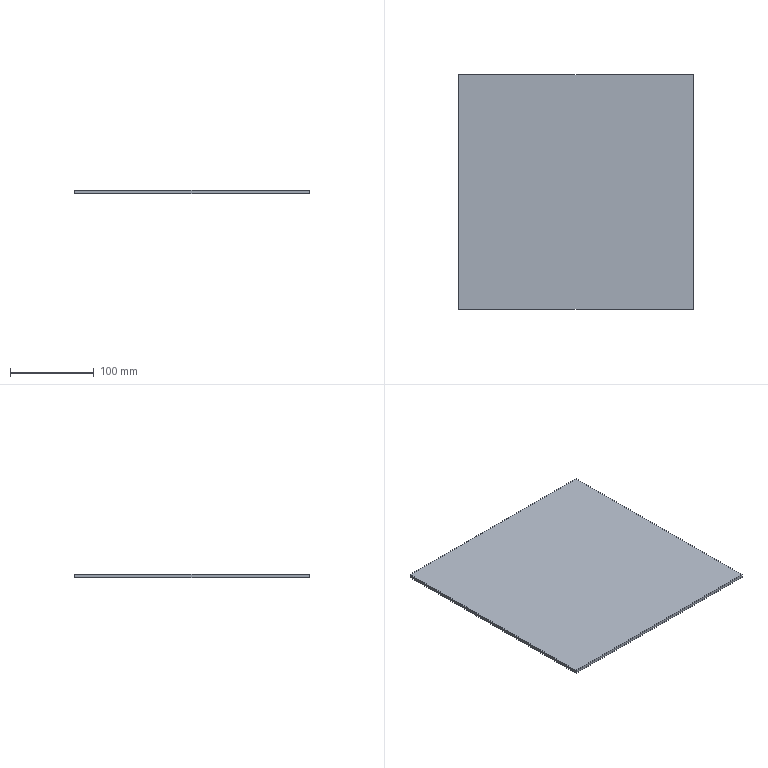Part | SolidWorks | features Extrusion 1 | 1 solid | 6 faces | box 280 x 280 x 4 mm | volume 313600 mm3 | plane 6
STEP:
#1=CARTESIAN_POINT('',(-140.,140.,2.));
#2=VERTEX_POINT('',#1);
#3=CARTESIAN_POINT('',(-140.,-140.,2.));
#4=VERTEX_POINT('',#3);
#5=CARTESIAN_POINT('',(-140.,140.,2.));
#6=DIRECTION('',(0.,-1.,0.));
#7=VECTOR('',#6,1000.);
#8=LINE('',#5,#7);
#9=EDGE_CURVE('',#2,#4,#8,.T.);
#10=ORIENTED_EDGE('',*,*,#9,.F.);
#11=CARTESIAN_POINT('',(-140.,140.,-2.));
#12=VERTEX_POINT('',#11);
#13=CARTESIAN_POINT('',(-140.,140.,-2.));
#14=DIRECTION('',(0.,0.,1.));
#15=VECTOR('',#14,1000.);
#16=LINE('',#13,#15);
#17=EDGE_CURVE('',#12,#2,#16,.T.);
#18=ORIENTED_EDGE('',*,*,#17,.F.);
#19=CARTESIAN_POINT('',(-140.,-140.,-2.));
#20=VERTEX_POINT('',#19);
#21=CARTESIAN_POINT('',(-140.,140.,-2.));
#22=DIRECTION('',(0.,-1.,0.));
#23=VECTOR('',#22,1000.);
#24=LINE('',#21,#23);
#25=EDGE_CURVE('',#12,#20,#24,.T.);
#26=ORIENTED_EDGE('',*,*,#25,.T.);
#27=CARTESIAN_POINT('',(-140.,-140.,-2.));
#28=DIRECTION('',(0.,0.,1.));
#29=VECTOR('',#28,1000.);
#30=LINE('',#27,#29);
#31=EDGE_CURVE('',#20,#4,#30,.T.);
#32=ORIENTED_EDGE('',*,*,#31,.T.);
#33=EDGE_LOOP('',(#10,#18,#26,#32));
#34=FACE_OUTER_BOUND('',#33,.T.);
#35=CARTESIAN_POINT('',(-140.,140.,-2.));
#36=DIRECTION('',(-1.,0.,0.));
#37=DIRECTION('',(0.,0.,1.));
#38=AXIS2_PLACEMENT_3D('',#35,#36,#37);
#39=PLANE('',#38);
#40=ADVANCED_FACE('',(#34),#39,.T.);
#41=CARTESIAN_POINT('',(140.,140.,2.));
#42=VERTEX_POINT('',#41);
#43=CARTESIAN_POINT('',(140.,140.,2.));
#44=DIRECTION('',(-1.,0.,0.));
#45=VECTOR('',#44,1000.);
#46=LINE('',#43,#45);
#47=EDGE_CURVE('',#42,#2,#46,.T.);
#48=ORIENTED_EDGE('',*,*,#47,.F.);
#49=CARTESIAN_POINT('',(140.,140.,-2.));
#50=VERTEX_POINT('',#49);
#51=CARTESIAN_POINT('',(140.,140.,-2.));
#52=DIRECTION('',(0.,0.,1.));
#53=VECTOR('',#52,1000.);
#54=LINE('',#51,#53);
#55=EDGE_CURVE('',#50,#42,#54,.T.);
#56=ORIENTED_EDGE('',*,*,#55,.F.);
#57=CARTESIAN_POINT('',(140.,140.,-2.));
#58=DIRECTION('',(-1.,0.,0.));
#59=VECTOR('',#58,1000.);
#60=LINE('',#57,#59);
#61=EDGE_CURVE('',#50,#12,#60,.T.);
#62=ORIENTED_EDGE('',*,*,#61,.T.);
#63=ORIENTED_EDGE('',*,*,#17,.T.);
#64=EDGE_LOOP('',(#48,#56,#62,#63));
#65=FACE_OUTER_BOUND('',#64,.T.);
#66=CARTESIAN_POINT('',(140.,140.,-2.));
#67=DIRECTION('',(0.,1.,0.));
#68=DIRECTION('',(0.,0.,1.));
#69=AXIS2_PLACEMENT_3D('',#66,#67,#68);
#70=PLANE('',#69);
#71=ADVANCED_FACE('',(#65),#70,.T.);
#72=CARTESIAN_POINT('',(140.,-140.,2.));
#73=VERTEX_POINT('',#72);
#74=CARTESIAN_POINT('',(140.,-140.,2.));
#75=DIRECTION('',(0.,1.,0.));
#76=VECTOR('',#75,1000.);
#77=LINE('',#74,#76);
#78=EDGE_CURVE('',#73,#42,#77,.T.);
#79=ORIENTED_EDGE('',*,*,#78,.F.);
#80=CARTESIAN_POINT('',(140.,-140.,-2.));
#81=VERTEX_POINT('',#80);
#82=CARTESIAN_POINT('',(140.,-140.,-2.));
#83=DIRECTION('',(0.,0.,1.));
#84=VECTOR('',#83,1000.);
#85=LINE('',#82,#84);
#86=EDGE_CURVE('',#81,#73,#85,.T.);
#87=ORIENTED_EDGE('',*,*,#86,.F.);
#88=CARTESIAN_POINT('',(140.,-140.,-2.));
#89=DIRECTION('',(0.,1.,0.));
#90=VECTOR('',#89,1000.);
#91=LINE('',#88,#90);
#92=EDGE_CURVE('',#81,#50,#91,.T.);
#93=ORIENTED_EDGE('',*,*,#92,.T.);
#94=ORIENTED_EDGE('',*,*,#55,.T.);
#95=EDGE_LOOP('',(#79,#87,#93,#94));
#96=FACE_OUTER_BOUND('',#95,.T.);
#97=CARTESIAN_POINT('',(140.,-140.,-2.));
#98=DIRECTION('',(1.,0.,0.));
#99=DIRECTION('',(0.,0.,-1.));
#100=AXIS2_PLACEMENT_3D('',#97,#98,#99);
#101=PLANE('',#100);
#102=ADVANCED_FACE('',(#96),#101,.T.);
#103=CARTESIAN_POINT('',(-140.,-140.,2.));
#104=DIRECTION('',(1.,0.,0.));
#105=VECTOR('',#104,1000.);
#106=LINE('',#103,#105);
#107=EDGE_CURVE('',#4,#73,#106,.T.);
#108=ORIENTED_EDGE('',*,*,#107,.F.);
#109=ORIENTED_EDGE('',*,*,#31,.F.);
#110=CARTESIAN_POINT('',(-140.,-140.,-2.));
#111=DIRECTION('',(1.,0.,0.));
#112=VECTOR('',#111,1000.);
#113=LINE('',#110,#112);
#114=EDGE_CURVE('',#20,#81,#113,.T.);
#115=ORIENTED_EDGE('',*,*,#114,.T.);
#116=ORIENTED_EDGE('',*,*,#86,.T.);
#117=EDGE_LOOP('',(#108,#109,#115,#116));
#118=FACE_OUTER_BOUND('',#117,.T.);
#119=CARTESIAN_POINT('',(-140.,-140.,-2.));
#120=DIRECTION('',(0.,-1.,0.));
#121=DIRECTION('',(0.,0.,-1.));
#122=AXIS2_PLACEMENT_3D('',#119,#120,#121);
#123=PLANE('',#122);
#124=ADVANCED_FACE('',(#118),#123,.T.);
#125=ORIENTED_EDGE('',*,*,#25,.F.);
#126=ORIENTED_EDGE('',*,*,#61,.F.);
#127=ORIENTED_EDGE('',*,*,#92,.F.);
#128=ORIENTED_EDGE('',*,*,#114,.F.);
#129=EDGE_LOOP('',(#125,#126,#127,#128));
#130=FACE_OUTER_BOUND('',#129,.T.);
#131=CARTESIAN_POINT('',(0.,0.,-2.));
#132=DIRECTION('',(0.,0.,1.));
#133=DIRECTION('',(1.,0.,0.));
#134=AXIS2_PLACEMENT_3D('',#131,#132,#133);
#135=PLANE('',#134);
#136=ADVANCED_FACE('',(#130),#135,.F.);
#137=ORIENTED_EDGE('',*,*,#9,.T.);
#138=ORIENTED_EDGE('',*,*,#107,.T.);
#139=ORIENTED_EDGE('',*,*,#78,.T.);
#140=ORIENTED_EDGE('',*,*,#47,.T.);
#141=EDGE_LOOP('',(#137,#138,#139,#140));
#142=FACE_OUTER_BOUND('',#141,.T.);
#143=CARTESIAN_POINT('',(0.,0.,2.));
#144=DIRECTION('',(0.,0.,1.));
#145=DIRECTION('',(1.,0.,0.));
#146=AXIS2_PLACEMENT_3D('',#143,#144,#145);
#147=PLANE('',#146);
#148=ADVANCED_FACE('',(#142),#147,.T.);
#149=CLOSED_SHELL('',(#40,#71,#102,#124,#136,#148));
#150=MANIFOLD_SOLID_BREP('',#149);
#151=CARTESIAN_POINT('',(0.,0.,0.));
#152=DIRECTION('',(0.,0.,1.));
#153=DIRECTION('',(1.,0.,0.));
#154=AXIS2_PLACEMENT_3D('',#151,#152,#153);
#155=(LENGTH_UNIT()NAMED_UNIT(*)SI_UNIT(.MILLI.,.METRE.));
#156=UNCERTAINTY_MEASURE_WITH_UNIT(LENGTH_MEASURE(0.00001),#155,'','');
#157=(NAMED_UNIT(*)PLANE_ANGLE_UNIT()SI_UNIT($,.RADIAN.));
#158=(NAMED_UNIT(*)SI_UNIT($,.STERADIAN.)SOLID_ANGLE_UNIT());
#159=(GEOMETRIC_REPRESENTATION_CONTEXT(3)GLOBAL_UNCERTAINTY_ASSIGNED_CONTEXT((#156))GLOBAL_UNIT_ASSIGNED_CONTEXT((#155,#157,#158))REPRESENTATION_CONTEXT('',''));
#160=ADVANCED_BREP_SHAPE_REPRESENTATION('',(#150,#154),#159);